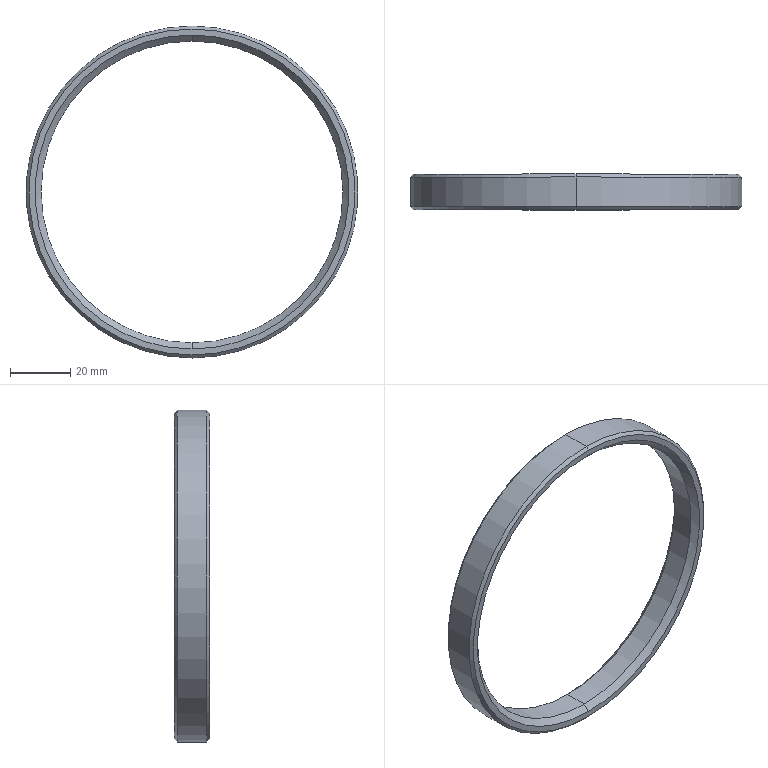Part | SolidWorks | features Chamfer 2, Extrusion 1 | 1 solid | 14 faces | box 110 x 11.75 x 110 mm | volume 17763 mm3 | cone 8 | cylinder 4 | plane 2 | commonest cylinder face diameters 100 x2 110 x2
STEP:
#1=CARTESIAN_POINT('',(0.,9.75,-50.));
#2=VERTEX_POINT('',#1);
#3=CARTESIAN_POINT('',(0.,9.75,50.));
#4=VERTEX_POINT('',#3);
#5=CARTESIAN_POINT('',(0.,9.75,0.));
#6=DIRECTION('',(0.,1.,0.));
#7=DIRECTION('',(0.,0.,1.));
#8=AXIS2_PLACEMENT_3D('',#5,#6,#7);
#9=CIRCLE('',#8,50.);
#10=EDGE_CURVE('',#2,#4,#9,.T.);
#11=ORIENTED_EDGE('',*,*,#10,.F.);
#12=CARTESIAN_POINT('',(0.,11.75,-52.));
#13=VERTEX_POINT('',#12);
#14=CARTESIAN_POINT('',(0.,9.75,-50.));
#15=DIRECTION('',(0.,0.7071,-0.7071));
#16=VECTOR('',#15,1000.);
#17=LINE('',#14,#16);
#18=EDGE_CURVE('',#2,#13,#17,.T.);
#19=ORIENTED_EDGE('',*,*,#18,.T.);
#20=CARTESIAN_POINT('',(0.,11.75,52.));
#21=VERTEX_POINT('',#20);
#22=CARTESIAN_POINT('',(0.,11.75,0.));
#23=DIRECTION('',(0.,-1.,0.));
#24=DIRECTION('',(0.,0.,1.));
#25=AXIS2_PLACEMENT_3D('',#22,#23,#24);
#26=CIRCLE('',#25,52.);
#27=EDGE_CURVE('',#21,#13,#26,.T.);
#28=ORIENTED_EDGE('',*,*,#27,.F.);
#29=CARTESIAN_POINT('',(0.,9.75,50.));
#30=DIRECTION('',(0.,0.7071,0.7071));
#31=VECTOR('',#30,1000.);
#32=LINE('',#29,#31);
#33=EDGE_CURVE('',#4,#21,#32,.T.);
#34=ORIENTED_EDGE('',*,*,#33,.F.);
#35=EDGE_LOOP('',(#11,#19,#28,#34));
#36=FACE_OUTER_BOUND('',#35,.T.);
#37=CARTESIAN_POINT('',(0.,9.75,0.));
#38=DIRECTION('',(0.,1.,0.));
#39=DIRECTION('',(0.,0.,1.));
#40=AXIS2_PLACEMENT_3D('',#37,#38,#39);
#41=CONICAL_SURFACE('',#40,50.,0.7854);
#42=ADVANCED_FACE('',(#36),#41,.F.);
#43=CARTESIAN_POINT('',(0.,2.,50.));
#44=VERTEX_POINT('',#43);
#45=CARTESIAN_POINT('',(0.,2.,-50.));
#46=VERTEX_POINT('',#45);
#47=CARTESIAN_POINT('',(0.,2.,0.));
#48=DIRECTION('',(0.,-1.,0.));
#49=DIRECTION('',(0.,0.,1.));
#50=AXIS2_PLACEMENT_3D('',#47,#48,#49);
#51=CIRCLE('',#50,50.);
#52=EDGE_CURVE('',#44,#46,#51,.T.);
#53=ORIENTED_EDGE('',*,*,#52,.F.);
#54=CARTESIAN_POINT('',(0.,0.,52.));
#55=VERTEX_POINT('',#54);
#56=CARTESIAN_POINT('',(0.,0.,52.));
#57=DIRECTION('',(0.,-0.7071,0.7071));
#58=VECTOR('',#57,1000.);
#59=LINE('',#56,#58);
#60=EDGE_CURVE('',#44,#55,#59,.T.);
#61=ORIENTED_EDGE('',*,*,#60,.T.);
#62=CARTESIAN_POINT('',(0.,0.,-52.));
#63=VERTEX_POINT('',#62);
#64=CARTESIAN_POINT('',(0.,0.,0.));
#65=DIRECTION('',(0.,1.,0.));
#66=DIRECTION('',(0.,0.,1.));
#67=AXIS2_PLACEMENT_3D('',#64,#65,#66);
#68=CIRCLE('',#67,52.);
#69=EDGE_CURVE('',#63,#55,#68,.T.);
#70=ORIENTED_EDGE('',*,*,#69,.F.);
#71=CARTESIAN_POINT('',(0.,0.,-52.));
#72=DIRECTION('',(0.,-0.7071,-0.7071));
#73=VECTOR('',#72,1000.);
#74=LINE('',#71,#73);
#75=EDGE_CURVE('',#46,#63,#74,.T.);
#76=ORIENTED_EDGE('',*,*,#75,.F.);
#77=EDGE_LOOP('',(#53,#61,#70,#76));
#78=FACE_OUTER_BOUND('',#77,.T.);
#79=CARTESIAN_POINT('',(0.,0.,0.));
#80=DIRECTION('',(0.,-1.,0.));
#81=DIRECTION('',(0.,0.,-1.));
#82=AXIS2_PLACEMENT_3D('',#79,#80,#81);
#83=CONICAL_SURFACE('',#82,52.,0.7854);
#84=ADVANCED_FACE('',(#78),#83,.F.);
#85=CARTESIAN_POINT('',(0.,11.75,54.));
#86=VERTEX_POINT('',#85);
#87=CARTESIAN_POINT('',(0.,11.75,-54.));
#88=VERTEX_POINT('',#87);
#89=CARTESIAN_POINT('',(0.,11.75,0.));
#90=DIRECTION('',(0.,1.,0.));
#91=DIRECTION('',(0.,0.,1.));
#92=AXIS2_PLACEMENT_3D('',#89,#90,#91);
#93=CIRCLE('',#92,54.);
#94=EDGE_CURVE('',#86,#88,#93,.T.);
#95=ORIENTED_EDGE('',*,*,#94,.F.);
#96=CARTESIAN_POINT('',(0.,10.75,55.));
#97=VERTEX_POINT('',#96);
#98=CARTESIAN_POINT('',(0.,11.75,54.));
#99=DIRECTION('',(0.,-0.7071,0.7071));
#100=VECTOR('',#99,1000.);
#101=LINE('',#98,#100);
#102=EDGE_CURVE('',#86,#97,#101,.T.);
#103=ORIENTED_EDGE('',*,*,#102,.T.);
#104=CARTESIAN_POINT('',(0.,10.75,-55.));
#105=VERTEX_POINT('',#104);
#106=CARTESIAN_POINT('',(0.,10.75,0.));
#107=DIRECTION('',(0.,-1.,0.));
#108=DIRECTION('',(0.,0.,1.));
#109=AXIS2_PLACEMENT_3D('',#106,#107,#108);
#110=CIRCLE('',#109,55.);
#111=EDGE_CURVE('',#105,#97,#110,.T.);
#112=ORIENTED_EDGE('',*,*,#111,.F.);
#113=CARTESIAN_POINT('',(0.,11.75,-54.));
#114=DIRECTION('',(0.,-0.7071,-0.7071));
#115=VECTOR('',#114,1000.);
#116=LINE('',#113,#115);
#117=EDGE_CURVE('',#88,#105,#116,.T.);
#118=ORIENTED_EDGE('',*,*,#117,.F.);
#119=EDGE_LOOP('',(#95,#103,#112,#118));
#120=FACE_OUTER_BOUND('',#119,.T.);
#121=CARTESIAN_POINT('',(0.,11.75,0.));
#122=DIRECTION('',(0.,-1.,0.));
#123=DIRECTION('',(0.,0.,-1.));
#124=AXIS2_PLACEMENT_3D('',#121,#122,#123);
#125=CONICAL_SURFACE('',#124,54.,0.7854);
#126=ADVANCED_FACE('',(#120),#125,.T.);
#127=CARTESIAN_POINT('',(0.,0.,-54.));
#128=VERTEX_POINT('',#127);
#129=CARTESIAN_POINT('',(0.,0.,54.));
#130=VERTEX_POINT('',#129);
#131=CARTESIAN_POINT('',(0.,0.,0.));
#132=DIRECTION('',(0.,-1.,0.));
#133=DIRECTION('',(0.,0.,1.));
#134=AXIS2_PLACEMENT_3D('',#131,#132,#133);
#135=CIRCLE('',#134,54.);
#136=EDGE_CURVE('',#128,#130,#135,.T.);
#137=ORIENTED_EDGE('',*,*,#136,.F.);
#138=CARTESIAN_POINT('',(0.,1.,-55.));
#139=VERTEX_POINT('',#138);
#140=CARTESIAN_POINT('',(0.,1.,-55.));
#141=DIRECTION('',(0.,0.7071,-0.7071));
#142=VECTOR('',#141,1000.);
#143=LINE('',#140,#142);
#144=EDGE_CURVE('',#128,#139,#143,.T.);
#145=ORIENTED_EDGE('',*,*,#144,.T.);
#146=CARTESIAN_POINT('',(0.,1.,55.));
#147=VERTEX_POINT('',#146);
#148=CARTESIAN_POINT('',(0.,1.,0.));
#149=DIRECTION('',(0.,1.,0.));
#150=DIRECTION('',(0.,0.,1.));
#151=AXIS2_PLACEMENT_3D('',#148,#149,#150);
#152=CIRCLE('',#151,55.);
#153=EDGE_CURVE('',#147,#139,#152,.T.);
#154=ORIENTED_EDGE('',*,*,#153,.F.);
#155=CARTESIAN_POINT('',(0.,1.,55.));
#156=DIRECTION('',(0.,0.7071,0.7071));
#157=VECTOR('',#156,1000.);
#158=LINE('',#155,#157);
#159=EDGE_CURVE('',#130,#147,#158,.T.);
#160=ORIENTED_EDGE('',*,*,#159,.F.);
#161=EDGE_LOOP('',(#137,#145,#154,#160));
#162=FACE_OUTER_BOUND('',#161,.T.);
#163=CARTESIAN_POINT('',(0.,1.,0.));
#164=DIRECTION('',(0.,1.,0.));
#165=DIRECTION('',(0.,0.,1.));
#166=AXIS2_PLACEMENT_3D('',#163,#164,#165);
#167=CONICAL_SURFACE('',#166,55.,0.7854);
#168=ADVANCED_FACE('',(#162),#167,.T.);
#169=ORIENTED_EDGE('',*,*,#10,.T.);
#170=CARTESIAN_POINT('',(0.,11.75,50.));
#171=DIRECTION('',(0.,-1.,0.));
#172=VECTOR('',#171,1000.);
#173=LINE('',#170,#172);
#174=EDGE_CURVE('',#4,#44,#173,.T.);
#175=ORIENTED_EDGE('',*,*,#174,.T.);
#176=ORIENTED_EDGE('',*,*,#52,.T.);
#177=CARTESIAN_POINT('',(0.,11.75,-50.));
#178=DIRECTION('',(0.,-1.,0.));
#179=VECTOR('',#178,1000.);
#180=LINE('',#177,#179);
#181=EDGE_CURVE('',#2,#46,#180,.T.);
#182=ORIENTED_EDGE('',*,*,#181,.F.);
#183=EDGE_LOOP('',(#169,#175,#176,#182));
#184=FACE_OUTER_BOUND('',#183,.T.);
#185=CARTESIAN_POINT('',(0.,11.75,0.));
#186=DIRECTION('',(0.,-1.,0.));
#187=DIRECTION('',(0.,0.,-1.));
#188=AXIS2_PLACEMENT_3D('',#185,#186,#187);
#189=CYLINDRICAL_SURFACE('',#188,50.);
#190=ADVANCED_FACE('',(#184),#189,.F.);
#191=ORIENTED_EDGE('',*,*,#111,.T.);
#192=CARTESIAN_POINT('',(0.,11.75,55.));
#193=DIRECTION('',(0.,-1.,0.));
#194=VECTOR('',#193,1000.);
#195=LINE('',#192,#194);
#196=EDGE_CURVE('',#97,#147,#195,.T.);
#197=ORIENTED_EDGE('',*,*,#196,.T.);
#198=ORIENTED_EDGE('',*,*,#153,.T.);
#199=CARTESIAN_POINT('',(0.,11.75,-55.));
#200=DIRECTION('',(0.,-1.,0.));
#201=VECTOR('',#200,1000.);
#202=LINE('',#199,#201);
#203=EDGE_CURVE('',#105,#139,#202,.T.);
#204=ORIENTED_EDGE('',*,*,#203,.F.);
#205=EDGE_LOOP('',(#191,#197,#198,#204));
#206=FACE_OUTER_BOUND('',#205,.T.);
#207=CARTESIAN_POINT('',(0.,11.75,0.));
#208=DIRECTION('',(0.,-1.,0.));
#209=DIRECTION('',(0.,0.,-1.));
#210=AXIS2_PLACEMENT_3D('',#207,#208,#209);
#211=CYLINDRICAL_SURFACE('',#210,55.);
#212=ADVANCED_FACE('',(#206),#211,.T.);
#213=ORIENTED_EDGE('',*,*,#27,.T.);
#214=CARTESIAN_POINT('',(0.,11.75,0.));
#215=DIRECTION('',(0.,-1.,0.));
#216=DIRECTION('',(0.,0.,1.));
#217=AXIS2_PLACEMENT_3D('',#214,#215,#216);
#218=CIRCLE('',#217,52.);
#219=EDGE_CURVE('',#13,#21,#218,.T.);
#220=ORIENTED_EDGE('',*,*,#219,.T.);
#221=EDGE_LOOP('',(#213,#220));
#222=FACE_BOUND('',#221,.T.);
#223=CARTESIAN_POINT('',(0.,11.75,0.));
#224=DIRECTION('',(0.,1.,0.));
#225=DIRECTION('',(0.,0.,1.));
#226=AXIS2_PLACEMENT_3D('',#223,#224,#225);
#227=CIRCLE('',#226,54.);
#228=EDGE_CURVE('',#88,#86,#227,.T.);
#229=ORIENTED_EDGE('',*,*,#228,.T.);
#230=ORIENTED_EDGE('',*,*,#94,.T.);
#231=EDGE_LOOP('',(#229,#230));
#232=FACE_OUTER_BOUND('',#231,.T.);
#233=CARTESIAN_POINT('',(0.,11.75,0.));
#234=DIRECTION('',(0.,1.,0.));
#235=DIRECTION('',(0.,0.,1.));
#236=AXIS2_PLACEMENT_3D('',#233,#234,#235);
#237=PLANE('',#236);
#238=ADVANCED_FACE('',(#222,#232),#237,.T.);
#239=ORIENTED_EDGE('',*,*,#69,.T.);
#240=CARTESIAN_POINT('',(0.,0.,0.));
#241=DIRECTION('',(0.,1.,0.));
#242=DIRECTION('',(0.,0.,1.));
#243=AXIS2_PLACEMENT_3D('',#240,#241,#242);
#244=CIRCLE('',#243,52.);
#245=EDGE_CURVE('',#55,#63,#244,.T.);
#246=ORIENTED_EDGE('',*,*,#245,.T.);
#247=EDGE_LOOP('',(#239,#246));
#248=FACE_BOUND('',#247,.T.);
#249=CARTESIAN_POINT('',(0.,0.,0.));
#250=DIRECTION('',(0.,-1.,0.));
#251=DIRECTION('',(0.,0.,1.));
#252=AXIS2_PLACEMENT_3D('',#249,#250,#251);
#253=CIRCLE('',#252,54.);
#254=EDGE_CURVE('',#130,#128,#253,.T.);
#255=ORIENTED_EDGE('',*,*,#254,.T.);
#256=ORIENTED_EDGE('',*,*,#136,.T.);
#257=EDGE_LOOP('',(#255,#256));
#258=FACE_OUTER_BOUND('',#257,.T.);
#259=CARTESIAN_POINT('',(0.,0.,0.));
#260=DIRECTION('',(0.,1.,0.));
#261=DIRECTION('',(0.,0.,1.));
#262=AXIS2_PLACEMENT_3D('',#259,#260,#261);
#263=PLANE('',#262);
#264=ADVANCED_FACE('',(#248,#258),#263,.F.);
#265=ORIENTED_EDGE('',*,*,#196,.F.);
#266=CARTESIAN_POINT('',(0.,10.75,0.));
#267=DIRECTION('',(0.,-1.,0.));
#268=DIRECTION('',(0.,0.,1.));
#269=AXIS2_PLACEMENT_3D('',#266,#267,#268);
#270=CIRCLE('',#269,55.);
#271=EDGE_CURVE('',#97,#105,#270,.T.);
#272=ORIENTED_EDGE('',*,*,#271,.T.);
#273=ORIENTED_EDGE('',*,*,#203,.T.);
#274=CARTESIAN_POINT('',(0.,1.,0.));
#275=DIRECTION('',(0.,1.,0.));
#276=DIRECTION('',(0.,0.,1.));
#277=AXIS2_PLACEMENT_3D('',#274,#275,#276);
#278=CIRCLE('',#277,55.);
#279=EDGE_CURVE('',#139,#147,#278,.T.);
#280=ORIENTED_EDGE('',*,*,#279,.T.);
#281=EDGE_LOOP('',(#265,#272,#273,#280));
#282=FACE_OUTER_BOUND('',#281,.T.);
#283=CARTESIAN_POINT('',(0.,11.75,0.));
#284=DIRECTION('',(0.,-1.,0.));
#285=DIRECTION('',(0.,0.,-1.));
#286=AXIS2_PLACEMENT_3D('',#283,#284,#285);
#287=CYLINDRICAL_SURFACE('',#286,55.);
#288=ADVANCED_FACE('',(#282),#287,.T.);
#289=ORIENTED_EDGE('',*,*,#174,.F.);
#290=CARTESIAN_POINT('',(0.,9.75,0.));
#291=DIRECTION('',(0.,1.,0.));
#292=DIRECTION('',(0.,0.,1.));
#293=AXIS2_PLACEMENT_3D('',#290,#291,#292);
#294=CIRCLE('',#293,50.);
#295=EDGE_CURVE('',#4,#2,#294,.T.);
#296=ORIENTED_EDGE('',*,*,#295,.T.);
#297=ORIENTED_EDGE('',*,*,#181,.T.);
#298=CARTESIAN_POINT('',(0.,2.,0.));
#299=DIRECTION('',(0.,-1.,0.));
#300=DIRECTION('',(0.,0.,1.));
#301=AXIS2_PLACEMENT_3D('',#298,#299,#300);
#302=CIRCLE('',#301,50.);
#303=EDGE_CURVE('',#46,#44,#302,.T.);
#304=ORIENTED_EDGE('',*,*,#303,.T.);
#305=EDGE_LOOP('',(#289,#296,#297,#304));
#306=FACE_OUTER_BOUND('',#305,.T.);
#307=CARTESIAN_POINT('',(0.,11.75,0.));
#308=DIRECTION('',(0.,-1.,0.));
#309=DIRECTION('',(0.,0.,-1.));
#310=AXIS2_PLACEMENT_3D('',#307,#308,#309);
#311=CYLINDRICAL_SURFACE('',#310,50.);
#312=ADVANCED_FACE('',(#306),#311,.F.);
#313=ORIENTED_EDGE('',*,*,#144,.F.);
#314=ORIENTED_EDGE('',*,*,#254,.F.);
#315=ORIENTED_EDGE('',*,*,#159,.T.);
#316=ORIENTED_EDGE('',*,*,#279,.F.);
#317=EDGE_LOOP('',(#313,#314,#315,#316));
#318=FACE_OUTER_BOUND('',#317,.T.);
#319=CARTESIAN_POINT('',(0.,1.,0.));
#320=DIRECTION('',(0.,1.,0.));
#321=DIRECTION('',(0.,0.,1.));
#322=AXIS2_PLACEMENT_3D('',#319,#320,#321);
#323=CONICAL_SURFACE('',#322,55.,0.7854);
#324=ADVANCED_FACE('',(#318),#323,.T.);
#325=ORIENTED_EDGE('',*,*,#102,.F.);
#326=ORIENTED_EDGE('',*,*,#228,.F.);
#327=ORIENTED_EDGE('',*,*,#117,.T.);
#328=ORIENTED_EDGE('',*,*,#271,.F.);
#329=EDGE_LOOP('',(#325,#326,#327,#328));
#330=FACE_OUTER_BOUND('',#329,.T.);
#331=CARTESIAN_POINT('',(0.,11.75,0.));
#332=DIRECTION('',(0.,-1.,0.));
#333=DIRECTION('',(0.,0.,-1.));
#334=AXIS2_PLACEMENT_3D('',#331,#332,#333);
#335=CONICAL_SURFACE('',#334,54.,0.7854);
#336=ADVANCED_FACE('',(#330),#335,.T.);
#337=ORIENTED_EDGE('',*,*,#60,.F.);
#338=ORIENTED_EDGE('',*,*,#303,.F.);
#339=ORIENTED_EDGE('',*,*,#75,.T.);
#340=ORIENTED_EDGE('',*,*,#245,.F.);
#341=EDGE_LOOP('',(#337,#338,#339,#340));
#342=FACE_OUTER_BOUND('',#341,.T.);
#343=CARTESIAN_POINT('',(0.,0.,0.));
#344=DIRECTION('',(0.,-1.,0.));
#345=DIRECTION('',(0.,0.,-1.));
#346=AXIS2_PLACEMENT_3D('',#343,#344,#345);
#347=CONICAL_SURFACE('',#346,52.,0.7854);
#348=ADVANCED_FACE('',(#342),#347,.F.);
#349=ORIENTED_EDGE('',*,*,#18,.F.);
#350=ORIENTED_EDGE('',*,*,#295,.F.);
#351=ORIENTED_EDGE('',*,*,#33,.T.);
#352=ORIENTED_EDGE('',*,*,#219,.F.);
#353=EDGE_LOOP('',(#349,#350,#351,#352));
#354=FACE_OUTER_BOUND('',#353,.T.);
#355=CARTESIAN_POINT('',(0.,9.75,0.));
#356=DIRECTION('',(0.,1.,0.));
#357=DIRECTION('',(0.,0.,1.));
#358=AXIS2_PLACEMENT_3D('',#355,#356,#357);
#359=CONICAL_SURFACE('',#358,50.,0.7854);
#360=ADVANCED_FACE('',(#354),#359,.F.);
#361=CLOSED_SHELL('',(#42,#84,#126,#168,#190,#212,#238,#264,#288,#312,#324,#336,#348,#360));
#362=MANIFOLD_SOLID_BREP('',#361);
#363=CARTESIAN_POINT('',(0.,0.,0.));
#364=DIRECTION('',(0.,0.,1.));
#365=DIRECTION('',(1.,0.,0.));
#366=AXIS2_PLACEMENT_3D('',#363,#364,#365);
#367=(LENGTH_UNIT()NAMED_UNIT(*)SI_UNIT(.MILLI.,.METRE.));
#368=UNCERTAINTY_MEASURE_WITH_UNIT(LENGTH_MEASURE(0.00001),#367,'','');
#369=(NAMED_UNIT(*)PLANE_ANGLE_UNIT()SI_UNIT($,.RADIAN.));
#370=(NAMED_UNIT(*)SI_UNIT($,.STERADIAN.)SOLID_ANGLE_UNIT());
#371=(GEOMETRIC_REPRESENTATION_CONTEXT(3)GLOBAL_UNCERTAINTY_ASSIGNED_CONTEXT((#368))GLOBAL_UNIT_ASSIGNED_CONTEXT((#367,#369,#370))REPRESENTATION_CONTEXT('',''));
#372=ADVANCED_BREP_SHAPE_REPRESENTATION('',(#362,#366),#371);